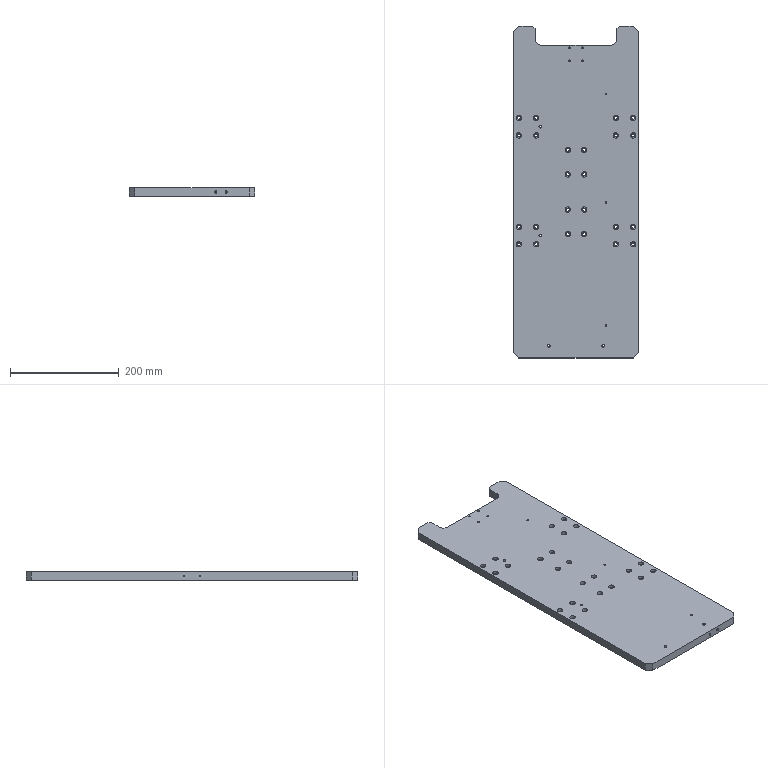Part | SolidWorks | features BaseBody 1 | 1 solid | 176 faces | box 230 x 610 x 15 mm | volume 2004849 mm3 | cylinder 128 | plane 40 | cone 8 | commonest cylinder face diameters 5.5 x48 10 x48 3.3 x14 5 x8 2.5 x4 4.2 x4